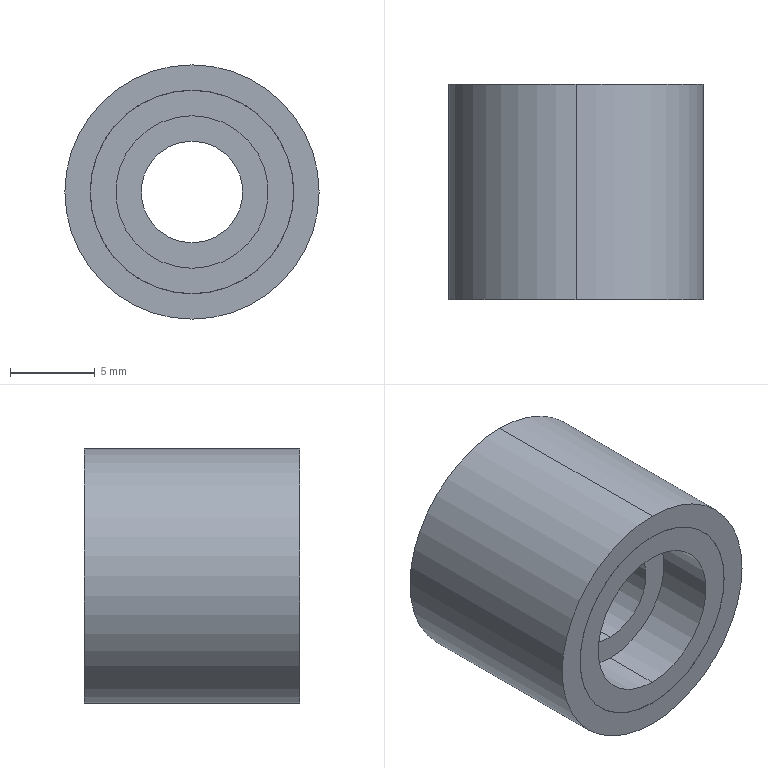Part | NX | features BREP 2 | 2 solids | 18 faces | box 15 x 12.7 x 15 mm | volume 1633 mm3 | cylinder 12 | plane 6 | commonest cylinder face diameters 9 x4 6 x2 12 x2 12.02 x2 15 x2
STEP:
#1=CARTESIAN_POINT('',(0.,6.35,-6.01));
#2=VERTEX_POINT('',#1);
#3=CARTESIAN_POINT('',(0.,-6.35,-6.01));
#4=VERTEX_POINT('',#3);
#5=CARTESIAN_POINT('',(0.,-6.35,-6.01));
#6=DIRECTION('',(0.,1.,0.));
#7=VECTOR('',#6,1000.);
#8=LINE('',#5,#7);
#9=EDGE_CURVE('',#2,#4,#8,.F.);
#10=ORIENTED_EDGE('',*,*,#9,.T.);
#11=CARTESIAN_POINT('',(0.,-6.35,6.01));
#12=VERTEX_POINT('',#11);
#13=CARTESIAN_POINT('',(0.,-6.35,0.));
#14=DIRECTION('',(0.,1.,0.));
#15=DIRECTION('',(1.,0.,0.));
#16=AXIS2_PLACEMENT_3D('',#13,#14,#15);
#17=CIRCLE('',#16,6.01);
#18=EDGE_CURVE('',#12,#4,#17,.T.);
#19=ORIENTED_EDGE('',*,*,#18,.F.);
#20=CARTESIAN_POINT('',(0.,6.35,6.01));
#21=VERTEX_POINT('',#20);
#22=CARTESIAN_POINT('',(0.,-6.35,6.01));
#23=DIRECTION('',(0.,1.,0.));
#24=VECTOR('',#23,1000.);
#25=LINE('',#22,#24);
#26=EDGE_CURVE('',#21,#12,#25,.F.);
#27=ORIENTED_EDGE('',*,*,#26,.F.);
#28=CARTESIAN_POINT('',(0.,6.35,0.));
#29=DIRECTION('',(0.,1.,0.));
#30=DIRECTION('',(1.,0.,0.));
#31=AXIS2_PLACEMENT_3D('',#28,#29,#30);
#32=CIRCLE('',#31,6.01);
#33=EDGE_CURVE('',#21,#2,#32,.T.);
#34=ORIENTED_EDGE('',*,*,#33,.T.);
#35=EDGE_LOOP('',(#10,#19,#27,#34));
#36=FACE_BOUND('',#35,.T.);
#37=CARTESIAN_POINT('',(0.,-6.35,0.));
#38=DIRECTION('',(0.,1.,0.));
#39=DIRECTION('',(0.,0.,1.));
#40=AXIS2_PLACEMENT_3D('',#37,#38,#39);
#41=CYLINDRICAL_SURFACE('',#40,6.01);
#42=ADVANCED_FACE('',(#36),#41,.F.);
#43=CARTESIAN_POINT('',(0.,-6.35,-7.5));
#44=VERTEX_POINT('',#43);
#45=CARTESIAN_POINT('',(0.,-6.35,7.5));
#46=VERTEX_POINT('',#45);
#47=CARTESIAN_POINT('',(0.,-6.35,0.));
#48=DIRECTION('',(0.,-1.,0.));
#49=DIRECTION('',(0.,0.,-1.));
#50=AXIS2_PLACEMENT_3D('',#47,#48,#49);
#51=CIRCLE('',#50,7.5);
#52=EDGE_CURVE('',#44,#46,#51,.T.);
#53=ORIENTED_EDGE('',*,*,#52,.T.);
#54=CARTESIAN_POINT('',(0.,-6.35,0.));
#55=DIRECTION('',(0.,-1.,0.));
#56=DIRECTION('',(0.,0.,-1.));
#57=AXIS2_PLACEMENT_3D('',#54,#55,#56);
#58=CIRCLE('',#57,7.5);
#59=EDGE_CURVE('',#46,#44,#58,.T.);
#60=ORIENTED_EDGE('',*,*,#59,.T.);
#61=EDGE_LOOP('',(#53,#60));
#62=FACE_BOUND('',#61,.T.);
#63=ORIENTED_EDGE('',*,*,#18,.T.);
#64=CARTESIAN_POINT('',(0.,-6.35,0.));
#65=DIRECTION('',(0.,1.,0.));
#66=DIRECTION('',(1.,0.,0.));
#67=AXIS2_PLACEMENT_3D('',#64,#65,#66);
#68=CIRCLE('',#67,6.01);
#69=EDGE_CURVE('',#4,#12,#68,.T.);
#70=ORIENTED_EDGE('',*,*,#69,.T.);
#71=EDGE_LOOP('',(#63,#70));
#72=FACE_BOUND('',#71,.T.);
#73=CARTESIAN_POINT('',(0.,-6.35,0.));
#74=DIRECTION('',(0.,1.,0.));
#75=DIRECTION('',(0.,0.,1.));
#76=AXIS2_PLACEMENT_3D('',#73,#74,#75);
#77=PLANE('',#76);
#78=ADVANCED_FACE('',(#62,#72),#77,.F.);
#79=CARTESIAN_POINT('',(0.,6.35,7.5));
#80=VERTEX_POINT('',#79);
#81=CARTESIAN_POINT('',(0.,0.,7.5));
#82=DIRECTION('',(0.,-1.,0.));
#83=VECTOR('',#82,1000.);
#84=LINE('',#81,#83);
#85=EDGE_CURVE('',#80,#46,#84,.T.);
#86=ORIENTED_EDGE('',*,*,#85,.F.);
#87=CARTESIAN_POINT('',(0.,6.35,-7.5));
#88=VERTEX_POINT('',#87);
#89=CARTESIAN_POINT('',(0.,6.35,0.));
#90=DIRECTION('',(0.,-1.,0.));
#91=DIRECTION('',(0.,0.,-1.));
#92=AXIS2_PLACEMENT_3D('',#89,#90,#91);
#93=CIRCLE('',#92,7.5);
#94=EDGE_CURVE('',#80,#88,#93,.T.);
#95=ORIENTED_EDGE('',*,*,#94,.T.);
#96=CARTESIAN_POINT('',(0.,0.,-7.5));
#97=DIRECTION('',(0.,-1.,0.));
#98=VECTOR('',#97,1000.);
#99=LINE('',#96,#98);
#100=EDGE_CURVE('',#88,#44,#99,.T.);
#101=ORIENTED_EDGE('',*,*,#100,.T.);
#102=ORIENTED_EDGE('',*,*,#59,.F.);
#103=EDGE_LOOP('',(#86,#95,#101,#102));
#104=FACE_BOUND('',#103,.T.);
#105=CARTESIAN_POINT('',(0.,0.,0.));
#106=DIRECTION('',(0.,-1.,0.));
#107=DIRECTION('',(0.,0.,-1.));
#108=AXIS2_PLACEMENT_3D('',#105,#106,#107);
#109=CYLINDRICAL_SURFACE('',#108,7.5);
#110=ADVANCED_FACE('',(#104),#109,.T.);
#111=CARTESIAN_POINT('',(0.,6.35,0.));
#112=DIRECTION('',(0.,-1.,0.));
#113=DIRECTION('',(0.,0.,-1.));
#114=AXIS2_PLACEMENT_3D('',#111,#112,#113);
#115=CIRCLE('',#114,7.5);
#116=EDGE_CURVE('',#88,#80,#115,.T.);
#117=ORIENTED_EDGE('',*,*,#116,.F.);
#118=ORIENTED_EDGE('',*,*,#94,.F.);
#119=EDGE_LOOP('',(#117,#118));
#120=FACE_BOUND('',#119,.T.);
#121=ORIENTED_EDGE('',*,*,#33,.F.);
#122=CARTESIAN_POINT('',(0.,6.35,0.));
#123=DIRECTION('',(0.,1.,0.));
#124=DIRECTION('',(1.,0.,0.));
#125=AXIS2_PLACEMENT_3D('',#122,#123,#124);
#126=CIRCLE('',#125,6.01);
#127=EDGE_CURVE('',#2,#21,#126,.T.);
#128=ORIENTED_EDGE('',*,*,#127,.F.);
#129=EDGE_LOOP('',(#121,#128));
#130=FACE_BOUND('',#129,.T.);
#131=CARTESIAN_POINT('',(0.,6.35,0.));
#132=DIRECTION('',(0.,1.,0.));
#133=DIRECTION('',(0.,0.,1.));
#134=AXIS2_PLACEMENT_3D('',#131,#132,#133);
#135=PLANE('',#134);
#136=ADVANCED_FACE('',(#120,#130),#135,.T.);
#137=ORIENTED_EDGE('',*,*,#116,.T.);
#138=ORIENTED_EDGE('',*,*,#85,.T.);
#139=ORIENTED_EDGE('',*,*,#52,.F.);
#140=ORIENTED_EDGE('',*,*,#100,.F.);
#141=EDGE_LOOP('',(#137,#138,#139,#140));
#142=FACE_BOUND('',#141,.T.);
#143=CARTESIAN_POINT('',(0.,0.,0.));
#144=DIRECTION('',(0.,-1.,0.));
#145=DIRECTION('',(0.,0.,-1.));
#146=AXIS2_PLACEMENT_3D('',#143,#144,#145);
#147=CYLINDRICAL_SURFACE('',#146,7.5);
#148=ADVANCED_FACE('',(#142),#147,.T.);
#149=ORIENTED_EDGE('',*,*,#69,.F.);
#150=ORIENTED_EDGE('',*,*,#9,.F.);
#151=ORIENTED_EDGE('',*,*,#127,.T.);
#152=ORIENTED_EDGE('',*,*,#26,.T.);
#153=EDGE_LOOP('',(#149,#150,#151,#152));
#154=FACE_BOUND('',#153,.T.);
#155=CARTESIAN_POINT('',(0.,-6.35,0.));
#156=DIRECTION('',(0.,1.,0.));
#157=DIRECTION('',(0.,0.,1.));
#158=AXIS2_PLACEMENT_3D('',#155,#156,#157);
#159=CYLINDRICAL_SURFACE('',#158,6.01);
#160=ADVANCED_FACE('',(#154),#159,.F.);
#161=CLOSED_SHELL('',(#42,#78,#110,#136,#148,#160));
#162=MANIFOLD_SOLID_BREP('',#161);
#163=CARTESIAN_POINT('',(0.,6.35,-6.));
#164=VERTEX_POINT('',#163);
#165=CARTESIAN_POINT('',(0.,-6.35,-6.));
#166=VERTEX_POINT('',#165);
#167=CARTESIAN_POINT('',(0.,-6.35,-6.));
#168=DIRECTION('',(0.,1.,0.));
#169=VECTOR('',#168,1000.);
#170=LINE('',#167,#169);
#171=EDGE_CURVE('',#164,#166,#170,.F.);
#172=ORIENTED_EDGE('',*,*,#171,.T.);
#173=CARTESIAN_POINT('',(0.,-6.35,6.));
#174=VERTEX_POINT('',#173);
#175=CARTESIAN_POINT('',(0.,-6.35,0.));
#176=DIRECTION('',(0.,1.,0.));
#177=DIRECTION('',(0.,0.,1.));
#178=AXIS2_PLACEMENT_3D('',#175,#176,#177);
#179=CIRCLE('',#178,6.);
#180=EDGE_CURVE('',#166,#174,#179,.T.);
#181=ORIENTED_EDGE('',*,*,#180,.T.);
#182=CARTESIAN_POINT('',(0.,6.35,6.));
#183=VERTEX_POINT('',#182);
#184=CARTESIAN_POINT('',(0.,-6.35,6.));
#185=DIRECTION('',(0.,1.,0.));
#186=VECTOR('',#185,1000.);
#187=LINE('',#184,#186);
#188=EDGE_CURVE('',#183,#174,#187,.F.);
#189=ORIENTED_EDGE('',*,*,#188,.F.);
#190=CARTESIAN_POINT('',(0.,6.35,0.));
#191=DIRECTION('',(0.,1.,0.));
#192=DIRECTION('',(0.,0.,1.));
#193=AXIS2_PLACEMENT_3D('',#190,#191,#192);
#194=CIRCLE('',#193,6.);
#195=EDGE_CURVE('',#164,#183,#194,.T.);
#196=ORIENTED_EDGE('',*,*,#195,.F.);
#197=EDGE_LOOP('',(#172,#181,#189,#196));
#198=FACE_BOUND('',#197,.T.);
#199=CARTESIAN_POINT('',(0.,-6.35,0.));
#200=DIRECTION('',(0.,1.,0.));
#201=DIRECTION('',(0.,0.,1.));
#202=AXIS2_PLACEMENT_3D('',#199,#200,#201);
#203=CYLINDRICAL_SURFACE('',#202,6.);
#204=ADVANCED_FACE('',(#198),#203,.T.);
#205=CARTESIAN_POINT('',(0.,2.85,-3.));
#206=VERTEX_POINT('',#205);
#207=CARTESIAN_POINT('',(0.,2.85,3.));
#208=VERTEX_POINT('',#207);
#209=CARTESIAN_POINT('',(0.,2.85,0.));
#210=DIRECTION('',(0.,-1.,0.));
#211=DIRECTION('',(0.,0.,-1.));
#212=AXIS2_PLACEMENT_3D('',#209,#210,#211);
#213=CIRCLE('',#212,3.);
#214=EDGE_CURVE('',#206,#208,#213,.T.);
#215=ORIENTED_EDGE('',*,*,#214,.T.);
#216=CARTESIAN_POINT('',(0.,2.85,0.));
#217=DIRECTION('',(0.,-1.,0.));
#218=DIRECTION('',(0.,0.,-1.));
#219=AXIS2_PLACEMENT_3D('',#216,#217,#218);
#220=CIRCLE('',#219,3.);
#221=EDGE_CURVE('',#208,#206,#220,.T.);
#222=ORIENTED_EDGE('',*,*,#221,.T.);
#223=EDGE_LOOP('',(#215,#222));
#224=FACE_BOUND('',#223,.T.);
#225=CARTESIAN_POINT('',(0.,2.85,-4.5));
#226=VERTEX_POINT('',#225);
#227=CARTESIAN_POINT('',(0.,2.85,4.5));
#228=VERTEX_POINT('',#227);
#229=CARTESIAN_POINT('',(0.,2.85,0.));
#230=DIRECTION('',(0.,-1.,0.));
#231=DIRECTION('',(0.,0.,-1.));
#232=AXIS2_PLACEMENT_3D('',#229,#230,#231);
#233=CIRCLE('',#232,4.5);
#234=EDGE_CURVE('',#226,#228,#233,.T.);
#235=ORIENTED_EDGE('',*,*,#234,.F.);
#236=CARTESIAN_POINT('',(0.,2.85,0.));
#237=DIRECTION('',(0.,-1.,0.));
#238=DIRECTION('',(0.,0.,-1.));
#239=AXIS2_PLACEMENT_3D('',#236,#237,#238);
#240=CIRCLE('',#239,4.5);
#241=EDGE_CURVE('',#228,#226,#240,.T.);
#242=ORIENTED_EDGE('',*,*,#241,.F.);
#243=EDGE_LOOP('',(#235,#242));
#244=FACE_BOUND('',#243,.T.);
#245=CARTESIAN_POINT('',(0.,2.85,0.));
#246=DIRECTION('',(0.,-1.,0.));
#247=DIRECTION('',(0.,0.,-1.));
#248=AXIS2_PLACEMENT_3D('',#245,#246,#247);
#249=PLANE('',#248);
#250=ADVANCED_FACE('',(#224,#244),#249,.F.);
#251=CARTESIAN_POINT('',(0.,-2.85,3.));
#252=VERTEX_POINT('',#251);
#253=CARTESIAN_POINT('',(0.,0.,3.));
#254=DIRECTION('',(0.,-1.,0.));
#255=VECTOR('',#254,1000.);
#256=LINE('',#253,#255);
#257=EDGE_CURVE('',#208,#252,#256,.T.);
#258=ORIENTED_EDGE('',*,*,#257,.F.);
#259=ORIENTED_EDGE('',*,*,#214,.F.);
#260=CARTESIAN_POINT('',(0.,-2.85,-3.));
#261=VERTEX_POINT('',#260);
#262=CARTESIAN_POINT('',(0.,0.,-3.));
#263=DIRECTION('',(0.,-1.,0.));
#264=VECTOR('',#263,1000.);
#265=LINE('',#262,#264);
#266=EDGE_CURVE('',#206,#261,#265,.T.);
#267=ORIENTED_EDGE('',*,*,#266,.T.);
#268=CARTESIAN_POINT('',(0.,-2.85,0.));
#269=DIRECTION('',(0.,-1.,0.));
#270=DIRECTION('',(0.,0.,-1.));
#271=AXIS2_PLACEMENT_3D('',#268,#269,#270);
#272=CIRCLE('',#271,3.);
#273=EDGE_CURVE('',#261,#252,#272,.T.);
#274=ORIENTED_EDGE('',*,*,#273,.T.);
#275=EDGE_LOOP('',(#258,#259,#267,#274));
#276=FACE_BOUND('',#275,.T.);
#277=CARTESIAN_POINT('',(0.,0.,0.));
#278=DIRECTION('',(0.,-1.,0.));
#279=DIRECTION('',(0.,0.,-1.));
#280=AXIS2_PLACEMENT_3D('',#277,#278,#279);
#281=CYLINDRICAL_SURFACE('',#280,3.);
#282=ADVANCED_FACE('',(#276),#281,.F.);
#283=ORIENTED_EDGE('',*,*,#273,.F.);
#284=CARTESIAN_POINT('',(0.,-2.85,0.));
#285=DIRECTION('',(0.,-1.,0.));
#286=DIRECTION('',(0.,0.,-1.));
#287=AXIS2_PLACEMENT_3D('',#284,#285,#286);
#288=CIRCLE('',#287,3.);
#289=EDGE_CURVE('',#252,#261,#288,.T.);
#290=ORIENTED_EDGE('',*,*,#289,.F.);
#291=EDGE_LOOP('',(#283,#290));
#292=FACE_BOUND('',#291,.T.);
#293=CARTESIAN_POINT('',(0.,-2.85,-4.5));
#294=VERTEX_POINT('',#293);
#295=CARTESIAN_POINT('',(0.,-2.85,4.5));
#296=VERTEX_POINT('',#295);
#297=CARTESIAN_POINT('',(0.,-2.85,0.));
#298=DIRECTION('',(0.,-1.,0.));
#299=DIRECTION('',(0.,0.,-1.));
#300=AXIS2_PLACEMENT_3D('',#297,#298,#299);
#301=CIRCLE('',#300,4.5);
#302=EDGE_CURVE('',#294,#296,#301,.T.);
#303=ORIENTED_EDGE('',*,*,#302,.T.);
#304=CARTESIAN_POINT('',(0.,-2.85,0.));
#305=DIRECTION('',(0.,-1.,0.));
#306=DIRECTION('',(0.,0.,-1.));
#307=AXIS2_PLACEMENT_3D('',#304,#305,#306);
#308=CIRCLE('',#307,4.5);
#309=EDGE_CURVE('',#296,#294,#308,.T.);
#310=ORIENTED_EDGE('',*,*,#309,.T.);
#311=EDGE_LOOP('',(#303,#310));
#312=FACE_BOUND('',#311,.T.);
#313=CARTESIAN_POINT('',(0.,-2.85,0.));
#314=DIRECTION('',(0.,-1.,0.));
#315=DIRECTION('',(0.,0.,-1.));
#316=AXIS2_PLACEMENT_3D('',#313,#314,#315);
#317=PLANE('',#316);
#318=ADVANCED_FACE('',(#292,#312),#317,.T.);
#319=CARTESIAN_POINT('',(0.,-6.35,4.5));
#320=VERTEX_POINT('',#319);
#321=CARTESIAN_POINT('',(0.,0.,4.5));
#322=DIRECTION('',(0.,-1.,0.));
#323=VECTOR('',#322,1000.);
#324=LINE('',#321,#323);
#325=EDGE_CURVE('',#296,#320,#324,.T.);
#326=ORIENTED_EDGE('',*,*,#325,.F.);
#327=ORIENTED_EDGE('',*,*,#302,.F.);
#328=CARTESIAN_POINT('',(0.,-6.35,-4.5));
#329=VERTEX_POINT('',#328);
#330=CARTESIAN_POINT('',(0.,0.,-4.5));
#331=DIRECTION('',(0.,-1.,0.));
#332=VECTOR('',#331,1000.);
#333=LINE('',#330,#332);
#334=EDGE_CURVE('',#294,#329,#333,.T.);
#335=ORIENTED_EDGE('',*,*,#334,.T.);
#336=CARTESIAN_POINT('',(0.,-6.35,0.));
#337=DIRECTION('',(0.,-1.,0.));
#338=DIRECTION('',(0.,0.,-1.));
#339=AXIS2_PLACEMENT_3D('',#336,#337,#338);
#340=CIRCLE('',#339,4.5);
#341=EDGE_CURVE('',#329,#320,#340,.T.);
#342=ORIENTED_EDGE('',*,*,#341,.T.);
#343=EDGE_LOOP('',(#326,#327,#335,#342));
#344=FACE_BOUND('',#343,.T.);
#345=CARTESIAN_POINT('',(0.,0.,0.));
#346=DIRECTION('',(0.,-1.,0.));
#347=DIRECTION('',(0.,0.,-1.));
#348=AXIS2_PLACEMENT_3D('',#345,#346,#347);
#349=CYLINDRICAL_SURFACE('',#348,4.5);
#350=ADVANCED_FACE('',(#344),#349,.F.);
#351=CARTESIAN_POINT('',(0.,6.35,4.5));
#352=VERTEX_POINT('',#351);
#353=CARTESIAN_POINT('',(0.,0.,4.5));
#354=DIRECTION('',(0.,-1.,0.));
#355=VECTOR('',#354,1000.);
#356=LINE('',#353,#355);
#357=EDGE_CURVE('',#352,#228,#356,.T.);
#358=ORIENTED_EDGE('',*,*,#357,.F.);
#359=CARTESIAN_POINT('',(0.,6.35,-4.5));
#360=VERTEX_POINT('',#359);
#361=CARTESIAN_POINT('',(0.,6.35,0.));
#362=DIRECTION('',(0.,-1.,0.));
#363=DIRECTION('',(0.,0.,-1.));
#364=AXIS2_PLACEMENT_3D('',#361,#362,#363);
#365=CIRCLE('',#364,4.5);
#366=EDGE_CURVE('',#360,#352,#365,.T.);
#367=ORIENTED_EDGE('',*,*,#366,.F.);
#368=CARTESIAN_POINT('',(0.,0.,-4.5));
#369=DIRECTION('',(0.,-1.,0.));
#370=VECTOR('',#369,1000.);
#371=LINE('',#368,#370);
#372=EDGE_CURVE('',#360,#226,#371,.T.);
#373=ORIENTED_EDGE('',*,*,#372,.T.);
#374=ORIENTED_EDGE('',*,*,#234,.T.);
#375=EDGE_LOOP('',(#358,#367,#373,#374));
#376=FACE_BOUND('',#375,.T.);
#377=CARTESIAN_POINT('',(0.,0.,0.));
#378=DIRECTION('',(0.,-1.,0.));
#379=DIRECTION('',(0.,0.,-1.));
#380=AXIS2_PLACEMENT_3D('',#377,#378,#379);
#381=CYLINDRICAL_SURFACE('',#380,4.5);
#382=ADVANCED_FACE('',(#376),#381,.F.);
#383=CARTESIAN_POINT('',(0.,-6.35,0.));
#384=DIRECTION('',(0.,1.,0.));
#385=DIRECTION('',(0.,0.,1.));
#386=AXIS2_PLACEMENT_3D('',#383,#384,#385);
#387=CIRCLE('',#386,6.);
#388=EDGE_CURVE('',#174,#166,#387,.T.);
#389=ORIENTED_EDGE('',*,*,#388,.F.);
#390=ORIENTED_EDGE('',*,*,#180,.F.);
#391=EDGE_LOOP('',(#389,#390));
#392=FACE_BOUND('',#391,.T.);
#393=ORIENTED_EDGE('',*,*,#341,.F.);
#394=CARTESIAN_POINT('',(0.,-6.35,0.));
#395=DIRECTION('',(0.,-1.,0.));
#396=DIRECTION('',(0.,0.,-1.));
#397=AXIS2_PLACEMENT_3D('',#394,#395,#396);
#398=CIRCLE('',#397,4.5);
#399=EDGE_CURVE('',#320,#329,#398,.T.);
#400=ORIENTED_EDGE('',*,*,#399,.F.);
#401=EDGE_LOOP('',(#393,#400));
#402=FACE_BOUND('',#401,.T.);
#403=CARTESIAN_POINT('',(0.,-6.35,0.));
#404=DIRECTION('',(0.,1.,0.));
#405=DIRECTION('',(0.,0.,1.));
#406=AXIS2_PLACEMENT_3D('',#403,#404,#405);
#407=PLANE('',#406);
#408=ADVANCED_FACE('',(#392,#402),#407,.F.);
#409=CARTESIAN_POINT('',(0.,6.35,0.));
#410=DIRECTION('',(0.,1.,0.));
#411=DIRECTION('',(0.,0.,1.));
#412=AXIS2_PLACEMENT_3D('',#409,#410,#411);
#413=CIRCLE('',#412,6.);
#414=EDGE_CURVE('',#183,#164,#413,.T.);
#415=ORIENTED_EDGE('',*,*,#414,.T.);
#416=ORIENTED_EDGE('',*,*,#195,.T.);
#417=EDGE_LOOP('',(#415,#416));
#418=FACE_BOUND('',#417,.T.);
#419=ORIENTED_EDGE('',*,*,#366,.T.);
#420=CARTESIAN_POINT('',(0.,6.35,0.));
#421=DIRECTION('',(0.,-1.,0.));
#422=DIRECTION('',(0.,0.,-1.));
#423=AXIS2_PLACEMENT_3D('',#420,#421,#422);
#424=CIRCLE('',#423,4.5);
#425=EDGE_CURVE('',#352,#360,#424,.T.);
#426=ORIENTED_EDGE('',*,*,#425,.T.);
#427=EDGE_LOOP('',(#419,#426));
#428=FACE_BOUND('',#427,.T.);
#429=CARTESIAN_POINT('',(0.,6.35,0.));
#430=DIRECTION('',(0.,1.,0.));
#431=DIRECTION('',(0.,0.,1.));
#432=AXIS2_PLACEMENT_3D('',#429,#430,#431);
#433=PLANE('',#432);
#434=ADVANCED_FACE('',(#418,#428),#433,.T.);
#435=ORIENTED_EDGE('',*,*,#425,.F.);
#436=ORIENTED_EDGE('',*,*,#357,.T.);
#437=ORIENTED_EDGE('',*,*,#241,.T.);
#438=ORIENTED_EDGE('',*,*,#372,.F.);
#439=EDGE_LOOP('',(#435,#436,#437,#438));
#440=FACE_BOUND('',#439,.T.);
#441=CARTESIAN_POINT('',(0.,0.,0.));
#442=DIRECTION('',(0.,-1.,0.));
#443=DIRECTION('',(0.,0.,-1.));
#444=AXIS2_PLACEMENT_3D('',#441,#442,#443);
#445=CYLINDRICAL_SURFACE('',#444,4.5);
#446=ADVANCED_FACE('',(#440),#445,.F.);
#447=ORIENTED_EDGE('',*,*,#309,.F.);
#448=ORIENTED_EDGE('',*,*,#325,.T.);
#449=ORIENTED_EDGE('',*,*,#399,.T.);
#450=ORIENTED_EDGE('',*,*,#334,.F.);
#451=EDGE_LOOP('',(#447,#448,#449,#450));
#452=FACE_BOUND('',#451,.T.);
#453=CARTESIAN_POINT('',(0.,0.,0.));
#454=DIRECTION('',(0.,-1.,0.));
#455=DIRECTION('',(0.,0.,-1.));
#456=AXIS2_PLACEMENT_3D('',#453,#454,#455);
#457=CYLINDRICAL_SURFACE('',#456,4.5);
#458=ADVANCED_FACE('',(#452),#457,.F.);
#459=ORIENTED_EDGE('',*,*,#221,.F.);
#460=ORIENTED_EDGE('',*,*,#257,.T.);
#461=ORIENTED_EDGE('',*,*,#289,.T.);
#462=ORIENTED_EDGE('',*,*,#266,.F.);
#463=EDGE_LOOP('',(#459,#460,#461,#462));
#464=FACE_BOUND('',#463,.T.);
#465=CARTESIAN_POINT('',(0.,0.,0.));
#466=DIRECTION('',(0.,-1.,0.));
#467=DIRECTION('',(0.,0.,-1.));
#468=AXIS2_PLACEMENT_3D('',#465,#466,#467);
#469=CYLINDRICAL_SURFACE('',#468,3.);
#470=ADVANCED_FACE('',(#464),#469,.F.);
#471=ORIENTED_EDGE('',*,*,#388,.T.);
#472=ORIENTED_EDGE('',*,*,#171,.F.);
#473=ORIENTED_EDGE('',*,*,#414,.F.);
#474=ORIENTED_EDGE('',*,*,#188,.T.);
#475=EDGE_LOOP('',(#471,#472,#473,#474));
#476=FACE_BOUND('',#475,.T.);
#477=CARTESIAN_POINT('',(0.,-6.35,0.));
#478=DIRECTION('',(0.,1.,0.));
#479=DIRECTION('',(0.,0.,1.));
#480=AXIS2_PLACEMENT_3D('',#477,#478,#479);
#481=CYLINDRICAL_SURFACE('',#480,6.);
#482=ADVANCED_FACE('',(#476),#481,.T.);
#483=CLOSED_SHELL('',(#204,#250,#282,#318,#350,#382,#408,#434,#446,#458,#470,#482));
#484=MANIFOLD_SOLID_BREP('',#483);
#485=(LENGTH_UNIT()NAMED_UNIT(*)SI_UNIT(.MILLI.,.METRE.));
#486=UNCERTAINTY_MEASURE_WITH_UNIT(LENGTH_MEASURE(0.00001),#485,'','');
#487=(NAMED_UNIT(*)PLANE_ANGLE_UNIT()SI_UNIT($,.RADIAN.));
#488=(NAMED_UNIT(*)SI_UNIT($,.STERADIAN.)SOLID_ANGLE_UNIT());
#489=(GEOMETRIC_REPRESENTATION_CONTEXT(3)GLOBAL_UNCERTAINTY_ASSIGNED_CONTEXT((#486))GLOBAL_UNIT_ASSIGNED_CONTEXT((#485,#487,#488))REPRESENTATION_CONTEXT('',''));
#490=ADVANCED_BREP_SHAPE_REPRESENTATION('',(#162,#484),#489);